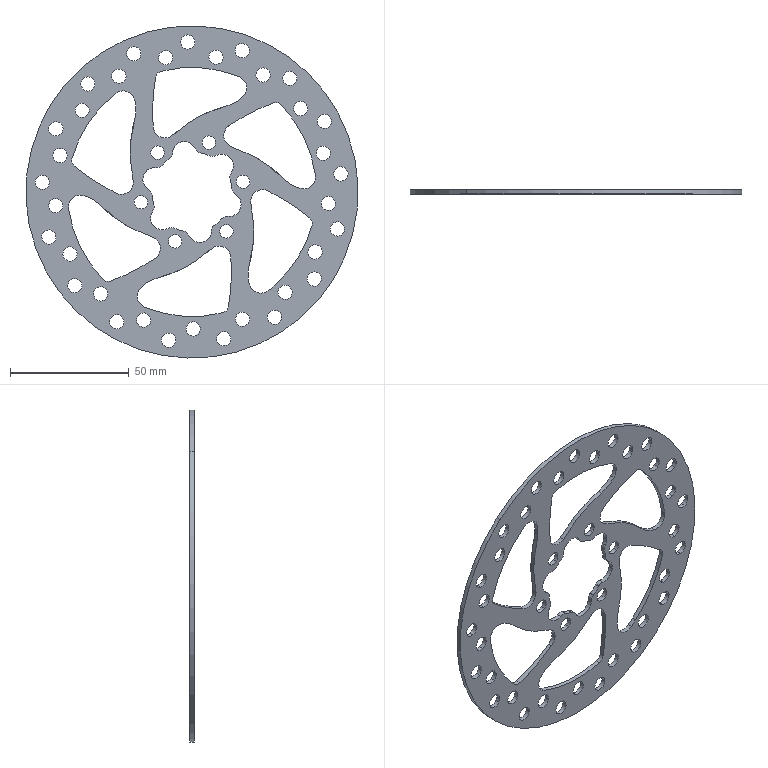Part | SolidWorks | features BaseBody 1 | 1 solid | 158 faces | box 140 x 1.86 x 140 mm | volume 15748 mm3 | cylinder 150 | spline 6 | plane 2 | commonest cylinder face diameters 6 x88 10 x22 5.7 x12 33.8 x7 105 x7 30 x6